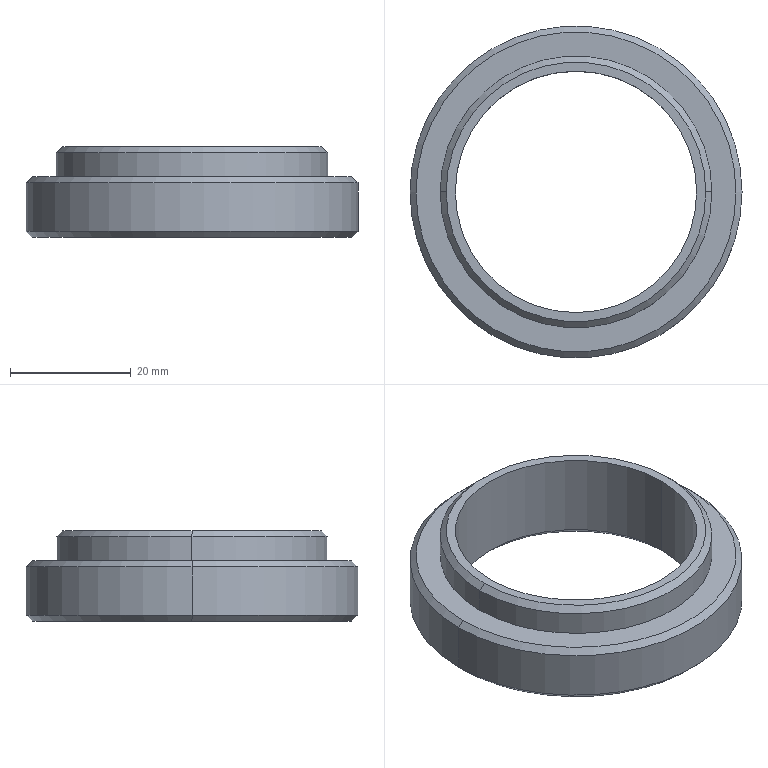Part | SolidWorks | features Chamfer 1, Extrusion 1, ICE 1 | 1 solid | 17 faces | box 55 x 55 x 15 mm | volume 12557 mm3 | cone 8 | cylinder 6 | plane 3 | commonest cylinder face diameters 40 x2 45 x2 55 x2
STEP:
#1=CARTESIAN_POINT('',(21.5,0.,15.));
#2=VERTEX_POINT('',#1);
#3=CARTESIAN_POINT('',(-21.5,0.,15.));
#4=VERTEX_POINT('',#3);
#5=CARTESIAN_POINT('',(0.,0.,15.));
#6=DIRECTION('',(0.,0.,1.));
#7=DIRECTION('',(1.,0.,0.));
#8=AXIS2_PLACEMENT_3D('',#5,#6,#7);
#9=CIRCLE('',#8,21.5);
#10=EDGE_CURVE('',#2,#4,#9,.T.);
#11=ORIENTED_EDGE('',*,*,#10,.F.);
#12=CARTESIAN_POINT('',(22.5,0.,14.));
#13=VERTEX_POINT('',#12);
#14=CARTESIAN_POINT('',(21.5,0.,15.));
#15=DIRECTION('',(0.7071,0.,-0.7071));
#16=VECTOR('',#15,1000.);
#17=LINE('',#14,#16);
#18=EDGE_CURVE('',#2,#13,#17,.T.);
#19=ORIENTED_EDGE('',*,*,#18,.T.);
#20=CARTESIAN_POINT('',(-22.5,0.,14.));
#21=VERTEX_POINT('',#20);
#22=CARTESIAN_POINT('',(0.,0.,14.));
#23=DIRECTION('',(0.,0.,-1.));
#24=DIRECTION('',(1.,0.,0.));
#25=AXIS2_PLACEMENT_3D('',#22,#23,#24);
#26=CIRCLE('',#25,22.5);
#27=EDGE_CURVE('',#21,#13,#26,.T.);
#28=ORIENTED_EDGE('',*,*,#27,.F.);
#29=CARTESIAN_POINT('',(-21.5,0.,15.));
#30=DIRECTION('',(-0.7071,0.,-0.7071));
#31=VECTOR('',#30,1000.);
#32=LINE('',#29,#31);
#33=EDGE_CURVE('',#4,#21,#32,.T.);
#34=ORIENTED_EDGE('',*,*,#33,.F.);
#35=EDGE_LOOP('',(#11,#19,#28,#34));
#36=FACE_OUTER_BOUND('',#35,.T.);
#37=CARTESIAN_POINT('',(0.,0.,15.));
#38=DIRECTION('',(0.,0.,-1.));
#39=DIRECTION('',(-1.,0.,0.));
#40=AXIS2_PLACEMENT_3D('',#37,#38,#39);
#41=CONICAL_SURFACE('',#40,21.5,0.7854);
#42=ADVANCED_FACE('',(#36),#41,.T.);
#43=CARTESIAN_POINT('',(26.5,0.,10.));
#44=VERTEX_POINT('',#43);
#45=CARTESIAN_POINT('',(-26.5,0.,10.));
#46=VERTEX_POINT('',#45);
#47=CARTESIAN_POINT('',(0.,0.,10.));
#48=DIRECTION('',(0.,0.,1.));
#49=DIRECTION('',(1.,0.,0.));
#50=AXIS2_PLACEMENT_3D('',#47,#48,#49);
#51=CIRCLE('',#50,26.5);
#52=EDGE_CURVE('',#44,#46,#51,.T.);
#53=ORIENTED_EDGE('',*,*,#52,.F.);
#54=CARTESIAN_POINT('',(27.5,0.,9.));
#55=VERTEX_POINT('',#54);
#56=CARTESIAN_POINT('',(26.5,0.,10.));
#57=DIRECTION('',(0.7071,0.,-0.7071));
#58=VECTOR('',#57,1000.);
#59=LINE('',#56,#58);
#60=EDGE_CURVE('',#44,#55,#59,.T.);
#61=ORIENTED_EDGE('',*,*,#60,.T.);
#62=CARTESIAN_POINT('',(-27.5,0.,9.));
#63=VERTEX_POINT('',#62);
#64=CARTESIAN_POINT('',(0.,0.,9.));
#65=DIRECTION('',(0.,0.,-1.));
#66=DIRECTION('',(1.,0.,0.));
#67=AXIS2_PLACEMENT_3D('',#64,#65,#66);
#68=CIRCLE('',#67,27.5);
#69=EDGE_CURVE('',#63,#55,#68,.T.);
#70=ORIENTED_EDGE('',*,*,#69,.F.);
#71=CARTESIAN_POINT('',(-26.5,0.,10.));
#72=DIRECTION('',(-0.7071,0.,-0.7071));
#73=VECTOR('',#72,1000.);
#74=LINE('',#71,#73);
#75=EDGE_CURVE('',#46,#63,#74,.T.);
#76=ORIENTED_EDGE('',*,*,#75,.F.);
#77=EDGE_LOOP('',(#53,#61,#70,#76));
#78=FACE_OUTER_BOUND('',#77,.T.);
#79=CARTESIAN_POINT('',(0.,0.,10.));
#80=DIRECTION('',(0.,0.,-1.));
#81=DIRECTION('',(-1.,0.,0.));
#82=AXIS2_PLACEMENT_3D('',#79,#80,#81);
#83=CONICAL_SURFACE('',#82,26.5,0.7854);
#84=ADVANCED_FACE('',(#78),#83,.T.);
#85=CARTESIAN_POINT('',(-26.5,0.,0.));
#86=VERTEX_POINT('',#85);
#87=CARTESIAN_POINT('',(26.5,0.,0.));
#88=VERTEX_POINT('',#87);
#89=CARTESIAN_POINT('',(0.,0.,0.));
#90=DIRECTION('',(0.,0.,-1.));
#91=DIRECTION('',(1.,0.,0.));
#92=AXIS2_PLACEMENT_3D('',#89,#90,#91);
#93=CIRCLE('',#92,26.5);
#94=EDGE_CURVE('',#86,#88,#93,.T.);
#95=ORIENTED_EDGE('',*,*,#94,.F.);
#96=CARTESIAN_POINT('',(-27.5,0.,1.));
#97=VERTEX_POINT('',#96);
#98=CARTESIAN_POINT('',(-27.5,0.,1.));
#99=DIRECTION('',(-0.7071,0.,0.7071));
#100=VECTOR('',#99,1000.);
#101=LINE('',#98,#100);
#102=EDGE_CURVE('',#86,#97,#101,.T.);
#103=ORIENTED_EDGE('',*,*,#102,.T.);
#104=CARTESIAN_POINT('',(27.5,0.,1.));
#105=VERTEX_POINT('',#104);
#106=CARTESIAN_POINT('',(0.,0.,1.));
#107=DIRECTION('',(0.,0.,1.));
#108=DIRECTION('',(1.,0.,0.));
#109=AXIS2_PLACEMENT_3D('',#106,#107,#108);
#110=CIRCLE('',#109,27.5);
#111=EDGE_CURVE('',#105,#97,#110,.T.);
#112=ORIENTED_EDGE('',*,*,#111,.F.);
#113=CARTESIAN_POINT('',(27.5,0.,1.));
#114=DIRECTION('',(0.7071,0.,0.7071));
#115=VECTOR('',#114,1000.);
#116=LINE('',#113,#115);
#117=EDGE_CURVE('',#88,#105,#116,.T.);
#118=ORIENTED_EDGE('',*,*,#117,.F.);
#119=EDGE_LOOP('',(#95,#103,#112,#118));
#120=FACE_OUTER_BOUND('',#119,.T.);
#121=CARTESIAN_POINT('',(0.,0.,1.));
#122=DIRECTION('',(0.,0.,1.));
#123=DIRECTION('',(1.,0.,0.));
#124=AXIS2_PLACEMENT_3D('',#121,#122,#123);
#125=CONICAL_SURFACE('',#124,27.5,0.7854);
#126=ADVANCED_FACE('',(#120),#125,.T.);
#127=CARTESIAN_POINT('',(20.,0.,1.));
#128=VERTEX_POINT('',#127);
#129=CARTESIAN_POINT('',(-20.,0.,1.));
#130=VERTEX_POINT('',#129);
#131=CARTESIAN_POINT('',(0.,0.,1.));
#132=DIRECTION('',(0.,0.,-1.));
#133=DIRECTION('',(1.,0.,0.));
#134=AXIS2_PLACEMENT_3D('',#131,#132,#133);
#135=CIRCLE('',#134,20.);
#136=EDGE_CURVE('',#128,#130,#135,.T.);
#137=ORIENTED_EDGE('',*,*,#136,.F.);
#138=CARTESIAN_POINT('',(21.,0.,0.));
#139=VERTEX_POINT('',#138);
#140=CARTESIAN_POINT('',(21.,0.,0.));
#141=DIRECTION('',(0.7071,0.,-0.7071));
#142=VECTOR('',#141,1000.);
#143=LINE('',#140,#142);
#144=EDGE_CURVE('',#128,#139,#143,.T.);
#145=ORIENTED_EDGE('',*,*,#144,.T.);
#146=CARTESIAN_POINT('',(-21.,0.,0.));
#147=VERTEX_POINT('',#146);
#148=CARTESIAN_POINT('',(0.,0.,0.));
#149=DIRECTION('',(0.,0.,1.));
#150=DIRECTION('',(1.,0.,0.));
#151=AXIS2_PLACEMENT_3D('',#148,#149,#150);
#152=CIRCLE('',#151,21.);
#153=EDGE_CURVE('',#147,#139,#152,.T.);
#154=ORIENTED_EDGE('',*,*,#153,.F.);
#155=CARTESIAN_POINT('',(-21.,0.,0.));
#156=DIRECTION('',(-0.7071,0.,-0.7071));
#157=VECTOR('',#156,1000.);
#158=LINE('',#155,#157);
#159=EDGE_CURVE('',#130,#147,#158,.T.);
#160=ORIENTED_EDGE('',*,*,#159,.F.);
#161=EDGE_LOOP('',(#137,#145,#154,#160));
#162=FACE_OUTER_BOUND('',#161,.T.);
#163=CARTESIAN_POINT('',(0.,0.,0.));
#164=DIRECTION('',(0.,0.,-1.));
#165=DIRECTION('',(-1.,0.,0.));
#166=AXIS2_PLACEMENT_3D('',#163,#164,#165);
#167=CONICAL_SURFACE('',#166,21.,0.7854);
#168=ADVANCED_FACE('',(#162),#167,.F.);
#169=CARTESIAN_POINT('',(22.5,0.,10.));
#170=VERTEX_POINT('',#169);
#171=CARTESIAN_POINT('',(-22.5,0.,10.));
#172=VERTEX_POINT('',#171);
#173=CARTESIAN_POINT('',(0.,0.,10.));
#174=DIRECTION('',(0.,0.,1.));
#175=DIRECTION('',(1.,0.,0.));
#176=AXIS2_PLACEMENT_3D('',#173,#174,#175);
#177=CIRCLE('',#176,22.5);
#178=EDGE_CURVE('',#170,#172,#177,.T.);
#179=ORIENTED_EDGE('',*,*,#178,.T.);
#180=CARTESIAN_POINT('',(-22.5,0.,10.));
#181=DIRECTION('',(0.,0.,1.));
#182=VECTOR('',#181,1000.);
#183=LINE('',#180,#182);
#184=EDGE_CURVE('',#172,#21,#183,.T.);
#185=ORIENTED_EDGE('',*,*,#184,.T.);
#186=ORIENTED_EDGE('',*,*,#27,.T.);
#187=CARTESIAN_POINT('',(22.5,0.,10.));
#188=DIRECTION('',(0.,0.,1.));
#189=VECTOR('',#188,1000.);
#190=LINE('',#187,#189);
#191=EDGE_CURVE('',#170,#13,#190,.T.);
#192=ORIENTED_EDGE('',*,*,#191,.F.);
#193=EDGE_LOOP('',(#179,#185,#186,#192));
#194=FACE_OUTER_BOUND('',#193,.T.);
#195=CARTESIAN_POINT('',(0.,0.,10.));
#196=DIRECTION('',(0.,0.,1.));
#197=DIRECTION('',(1.,0.,0.));
#198=AXIS2_PLACEMENT_3D('',#195,#196,#197);
#199=CYLINDRICAL_SURFACE('',#198,22.5);
#200=ADVANCED_FACE('',(#194),#199,.T.);
#201=CARTESIAN_POINT('',(-20.,0.,15.));
#202=VERTEX_POINT('',#201);
#203=CARTESIAN_POINT('',(20.,0.,15.));
#204=VERTEX_POINT('',#203);
#205=CARTESIAN_POINT('',(0.,0.,15.));
#206=DIRECTION('',(0.,0.,1.));
#207=DIRECTION('',(1.,0.,0.));
#208=AXIS2_PLACEMENT_3D('',#205,#206,#207);
#209=CIRCLE('',#208,20.);
#210=EDGE_CURVE('',#202,#204,#209,.T.);
#211=ORIENTED_EDGE('',*,*,#210,.T.);
#212=CARTESIAN_POINT('',(20.,0.,15.));
#213=DIRECTION('',(0.,0.,-1.));
#214=VECTOR('',#213,1000.);
#215=LINE('',#212,#214);
#216=EDGE_CURVE('',#204,#128,#215,.T.);
#217=ORIENTED_EDGE('',*,*,#216,.T.);
#218=ORIENTED_EDGE('',*,*,#136,.T.);
#219=CARTESIAN_POINT('',(-20.,0.,15.));
#220=DIRECTION('',(0.,0.,-1.));
#221=VECTOR('',#220,1000.);
#222=LINE('',#219,#221);
#223=EDGE_CURVE('',#202,#130,#222,.T.);
#224=ORIENTED_EDGE('',*,*,#223,.F.);
#225=EDGE_LOOP('',(#211,#217,#218,#224));
#226=FACE_OUTER_BOUND('',#225,.T.);
#227=CARTESIAN_POINT('',(0.,0.,15.));
#228=DIRECTION('',(0.,0.,-1.));
#229=DIRECTION('',(-1.,0.,0.));
#230=AXIS2_PLACEMENT_3D('',#227,#228,#229);
#231=CYLINDRICAL_SURFACE('',#230,20.);
#232=ADVANCED_FACE('',(#226),#231,.F.);
#233=ORIENTED_EDGE('',*,*,#69,.T.);
#234=CARTESIAN_POINT('',(27.5,0.,15.));
#235=DIRECTION('',(0.,0.,-1.));
#236=VECTOR('',#235,1000.);
#237=LINE('',#234,#236);
#238=EDGE_CURVE('',#55,#105,#237,.T.);
#239=ORIENTED_EDGE('',*,*,#238,.T.);
#240=ORIENTED_EDGE('',*,*,#111,.T.);
#241=CARTESIAN_POINT('',(-27.5,0.,15.));
#242=DIRECTION('',(0.,0.,-1.));
#243=VECTOR('',#242,1000.);
#244=LINE('',#241,#243);
#245=EDGE_CURVE('',#63,#97,#244,.T.);
#246=ORIENTED_EDGE('',*,*,#245,.F.);
#247=EDGE_LOOP('',(#233,#239,#240,#246));
#248=FACE_OUTER_BOUND('',#247,.T.);
#249=CARTESIAN_POINT('',(0.,0.,15.));
#250=DIRECTION('',(0.,0.,-1.));
#251=DIRECTION('',(-1.,0.,0.));
#252=AXIS2_PLACEMENT_3D('',#249,#250,#251);
#253=CYLINDRICAL_SURFACE('',#252,27.5);
#254=ADVANCED_FACE('',(#248),#253,.T.);
#255=CARTESIAN_POINT('',(0.,0.,15.));
#256=DIRECTION('',(0.,0.,1.));
#257=DIRECTION('',(1.,0.,0.));
#258=AXIS2_PLACEMENT_3D('',#255,#256,#257);
#259=CIRCLE('',#258,21.5);
#260=EDGE_CURVE('',#4,#2,#259,.T.);
#261=ORIENTED_EDGE('',*,*,#260,.T.);
#262=ORIENTED_EDGE('',*,*,#10,.T.);
#263=EDGE_LOOP('',(#261,#262));
#264=FACE_OUTER_BOUND('',#263,.T.);
#265=ORIENTED_EDGE('',*,*,#210,.F.);
#266=CARTESIAN_POINT('',(0.,0.,15.));
#267=DIRECTION('',(0.,0.,1.));
#268=DIRECTION('',(1.,0.,0.));
#269=AXIS2_PLACEMENT_3D('',#266,#267,#268);
#270=CIRCLE('',#269,20.);
#271=EDGE_CURVE('',#204,#202,#270,.T.);
#272=ORIENTED_EDGE('',*,*,#271,.F.);
#273=EDGE_LOOP('',(#265,#272));
#274=FACE_BOUND('',#273,.T.);
#275=CARTESIAN_POINT('',(0.,0.,15.));
#276=DIRECTION('',(0.,0.,1.));
#277=DIRECTION('',(1.,0.,0.));
#278=AXIS2_PLACEMENT_3D('',#275,#276,#277);
#279=PLANE('',#278);
#280=ADVANCED_FACE('',(#264,#274),#279,.T.);
#281=ORIENTED_EDGE('',*,*,#238,.F.);
#282=CARTESIAN_POINT('',(0.,0.,9.));
#283=DIRECTION('',(0.,0.,-1.));
#284=DIRECTION('',(1.,0.,0.));
#285=AXIS2_PLACEMENT_3D('',#282,#283,#284);
#286=CIRCLE('',#285,27.5);
#287=EDGE_CURVE('',#55,#63,#286,.T.);
#288=ORIENTED_EDGE('',*,*,#287,.T.);
#289=ORIENTED_EDGE('',*,*,#245,.T.);
#290=CARTESIAN_POINT('',(0.,0.,1.));
#291=DIRECTION('',(0.,0.,1.));
#292=DIRECTION('',(1.,0.,0.));
#293=AXIS2_PLACEMENT_3D('',#290,#291,#292);
#294=CIRCLE('',#293,27.5);
#295=EDGE_CURVE('',#97,#105,#294,.T.);
#296=ORIENTED_EDGE('',*,*,#295,.T.);
#297=EDGE_LOOP('',(#281,#288,#289,#296));
#298=FACE_OUTER_BOUND('',#297,.T.);
#299=CARTESIAN_POINT('',(0.,0.,15.));
#300=DIRECTION('',(0.,0.,-1.));
#301=DIRECTION('',(-1.,0.,0.));
#302=AXIS2_PLACEMENT_3D('',#299,#300,#301);
#303=CYLINDRICAL_SURFACE('',#302,27.5);
#304=ADVANCED_FACE('',(#298),#303,.T.);
#305=ORIENTED_EDGE('',*,*,#153,.T.);
#306=CARTESIAN_POINT('',(0.,0.,0.));
#307=DIRECTION('',(0.,0.,1.));
#308=DIRECTION('',(1.,0.,0.));
#309=AXIS2_PLACEMENT_3D('',#306,#307,#308);
#310=CIRCLE('',#309,21.);
#311=EDGE_CURVE('',#139,#147,#310,.T.);
#312=ORIENTED_EDGE('',*,*,#311,.T.);
#313=EDGE_LOOP('',(#305,#312));
#314=FACE_BOUND('',#313,.T.);
#315=CARTESIAN_POINT('',(0.,0.,0.));
#316=DIRECTION('',(0.,0.,-1.));
#317=DIRECTION('',(1.,0.,0.));
#318=AXIS2_PLACEMENT_3D('',#315,#316,#317);
#319=CIRCLE('',#318,26.5);
#320=EDGE_CURVE('',#88,#86,#319,.T.);
#321=ORIENTED_EDGE('',*,*,#320,.T.);
#322=ORIENTED_EDGE('',*,*,#94,.T.);
#323=EDGE_LOOP('',(#321,#322));
#324=FACE_OUTER_BOUND('',#323,.T.);
#325=CARTESIAN_POINT('',(0.,0.,0.));
#326=DIRECTION('',(0.,0.,1.));
#327=DIRECTION('',(1.,0.,0.));
#328=AXIS2_PLACEMENT_3D('',#325,#326,#327);
#329=PLANE('',#328);
#330=ADVANCED_FACE('',(#314,#324),#329,.F.);
#331=ORIENTED_EDGE('',*,*,#216,.F.);
#332=ORIENTED_EDGE('',*,*,#271,.T.);
#333=ORIENTED_EDGE('',*,*,#223,.T.);
#334=CARTESIAN_POINT('',(0.,0.,1.));
#335=DIRECTION('',(0.,0.,-1.));
#336=DIRECTION('',(1.,0.,0.));
#337=AXIS2_PLACEMENT_3D('',#334,#335,#336);
#338=CIRCLE('',#337,20.);
#339=EDGE_CURVE('',#130,#128,#338,.T.);
#340=ORIENTED_EDGE('',*,*,#339,.T.);
#341=EDGE_LOOP('',(#331,#332,#333,#340));
#342=FACE_OUTER_BOUND('',#341,.T.);
#343=CARTESIAN_POINT('',(0.,0.,15.));
#344=DIRECTION('',(0.,0.,-1.));
#345=DIRECTION('',(-1.,0.,0.));
#346=AXIS2_PLACEMENT_3D('',#343,#344,#345);
#347=CYLINDRICAL_SURFACE('',#346,20.);
#348=ADVANCED_FACE('',(#342),#347,.F.);
#349=CARTESIAN_POINT('',(0.,0.,10.));
#350=DIRECTION('',(0.,0.,1.));
#351=DIRECTION('',(1.,0.,0.));
#352=AXIS2_PLACEMENT_3D('',#349,#350,#351);
#353=CIRCLE('',#352,26.5);
#354=EDGE_CURVE('',#46,#44,#353,.T.);
#355=ORIENTED_EDGE('',*,*,#354,.T.);
#356=ORIENTED_EDGE('',*,*,#52,.T.);
#357=EDGE_LOOP('',(#355,#356));
#358=FACE_OUTER_BOUND('',#357,.T.);
#359=ORIENTED_EDGE('',*,*,#178,.F.);
#360=CARTESIAN_POINT('',(0.,0.,10.));
#361=DIRECTION('',(0.,0.,1.));
#362=DIRECTION('',(1.,0.,0.));
#363=AXIS2_PLACEMENT_3D('',#360,#361,#362);
#364=CIRCLE('',#363,22.5);
#365=EDGE_CURVE('',#172,#170,#364,.T.);
#366=ORIENTED_EDGE('',*,*,#365,.F.);
#367=EDGE_LOOP('',(#359,#366));
#368=FACE_BOUND('',#367,.T.);
#369=CARTESIAN_POINT('',(0.,0.,10.));
#370=DIRECTION('',(0.,0.,1.));
#371=DIRECTION('',(1.,0.,0.));
#372=AXIS2_PLACEMENT_3D('',#369,#370,#371);
#373=PLANE('',#372);
#374=ADVANCED_FACE('',(#358,#368),#373,.T.);
#375=ORIENTED_EDGE('',*,*,#184,.F.);
#376=ORIENTED_EDGE('',*,*,#365,.T.);
#377=ORIENTED_EDGE('',*,*,#191,.T.);
#378=CARTESIAN_POINT('',(0.,0.,14.));
#379=DIRECTION('',(0.,0.,-1.));
#380=DIRECTION('',(1.,0.,0.));
#381=AXIS2_PLACEMENT_3D('',#378,#379,#380);
#382=CIRCLE('',#381,22.5);
#383=EDGE_CURVE('',#13,#21,#382,.T.);
#384=ORIENTED_EDGE('',*,*,#383,.T.);
#385=EDGE_LOOP('',(#375,#376,#377,#384));
#386=FACE_OUTER_BOUND('',#385,.T.);
#387=CARTESIAN_POINT('',(0.,0.,10.));
#388=DIRECTION('',(0.,0.,1.));
#389=DIRECTION('',(1.,0.,0.));
#390=AXIS2_PLACEMENT_3D('',#387,#388,#389);
#391=CYLINDRICAL_SURFACE('',#390,22.5);
#392=ADVANCED_FACE('',(#386),#391,.T.);
#393=ORIENTED_EDGE('',*,*,#144,.F.);
#394=ORIENTED_EDGE('',*,*,#339,.F.);
#395=ORIENTED_EDGE('',*,*,#159,.T.);
#396=ORIENTED_EDGE('',*,*,#311,.F.);
#397=EDGE_LOOP('',(#393,#394,#395,#396));
#398=FACE_OUTER_BOUND('',#397,.T.);
#399=CARTESIAN_POINT('',(0.,0.,0.));
#400=DIRECTION('',(0.,0.,-1.));
#401=DIRECTION('',(-1.,0.,0.));
#402=AXIS2_PLACEMENT_3D('',#399,#400,#401);
#403=CONICAL_SURFACE('',#402,21.,0.7854);
#404=ADVANCED_FACE('',(#398),#403,.F.);
#405=ORIENTED_EDGE('',*,*,#102,.F.);
#406=ORIENTED_EDGE('',*,*,#320,.F.);
#407=ORIENTED_EDGE('',*,*,#117,.T.);
#408=ORIENTED_EDGE('',*,*,#295,.F.);
#409=EDGE_LOOP('',(#405,#406,#407,#408));
#410=FACE_OUTER_BOUND('',#409,.T.);
#411=CARTESIAN_POINT('',(0.,0.,1.));
#412=DIRECTION('',(0.,0.,1.));
#413=DIRECTION('',(1.,0.,0.));
#414=AXIS2_PLACEMENT_3D('',#411,#412,#413);
#415=CONICAL_SURFACE('',#414,27.5,0.7854);
#416=ADVANCED_FACE('',(#410),#415,.T.);
#417=ORIENTED_EDGE('',*,*,#60,.F.);
#418=ORIENTED_EDGE('',*,*,#354,.F.);
#419=ORIENTED_EDGE('',*,*,#75,.T.);
#420=ORIENTED_EDGE('',*,*,#287,.F.);
#421=EDGE_LOOP('',(#417,#418,#419,#420));
#422=FACE_OUTER_BOUND('',#421,.T.);
#423=CARTESIAN_POINT('',(0.,0.,10.));
#424=DIRECTION('',(0.,0.,-1.));
#425=DIRECTION('',(-1.,0.,0.));
#426=AXIS2_PLACEMENT_3D('',#423,#424,#425);
#427=CONICAL_SURFACE('',#426,26.5,0.7854);
#428=ADVANCED_FACE('',(#422),#427,.T.);
#429=ORIENTED_EDGE('',*,*,#18,.F.);
#430=ORIENTED_EDGE('',*,*,#260,.F.);
#431=ORIENTED_EDGE('',*,*,#33,.T.);
#432=ORIENTED_EDGE('',*,*,#383,.F.);
#433=EDGE_LOOP('',(#429,#430,#431,#432));
#434=FACE_OUTER_BOUND('',#433,.T.);
#435=CARTESIAN_POINT('',(0.,0.,15.));
#436=DIRECTION('',(0.,0.,-1.));
#437=DIRECTION('',(-1.,0.,0.));
#438=AXIS2_PLACEMENT_3D('',#435,#436,#437);
#439=CONICAL_SURFACE('',#438,21.5,0.7854);
#440=ADVANCED_FACE('',(#434),#439,.T.);
#441=CLOSED_SHELL('',(#42,#84,#126,#168,#200,#232,#254,#280,#304,#330,#348,#374,#392,#404,#416,#428,#440));
#442=MANIFOLD_SOLID_BREP('',#441);
#443=CARTESIAN_POINT('',(0.,0.,0.));
#444=DIRECTION('',(0.,0.,1.));
#445=DIRECTION('',(1.,0.,0.));
#446=AXIS2_PLACEMENT_3D('',#443,#444,#445);
#447=(LENGTH_UNIT()NAMED_UNIT(*)SI_UNIT(.MILLI.,.METRE.));
#448=UNCERTAINTY_MEASURE_WITH_UNIT(LENGTH_MEASURE(0.00001),#447,'','');
#449=(NAMED_UNIT(*)PLANE_ANGLE_UNIT()SI_UNIT($,.RADIAN.));
#450=(NAMED_UNIT(*)SI_UNIT($,.STERADIAN.)SOLID_ANGLE_UNIT());
#451=(GEOMETRIC_REPRESENTATION_CONTEXT(3)GLOBAL_UNCERTAINTY_ASSIGNED_CONTEXT((#448))GLOBAL_UNIT_ASSIGNED_CONTEXT((#447,#449,#450))REPRESENTATION_CONTEXT('',''));
#452=ADVANCED_BREP_SHAPE_REPRESENTATION('',(#442,#446),#451);